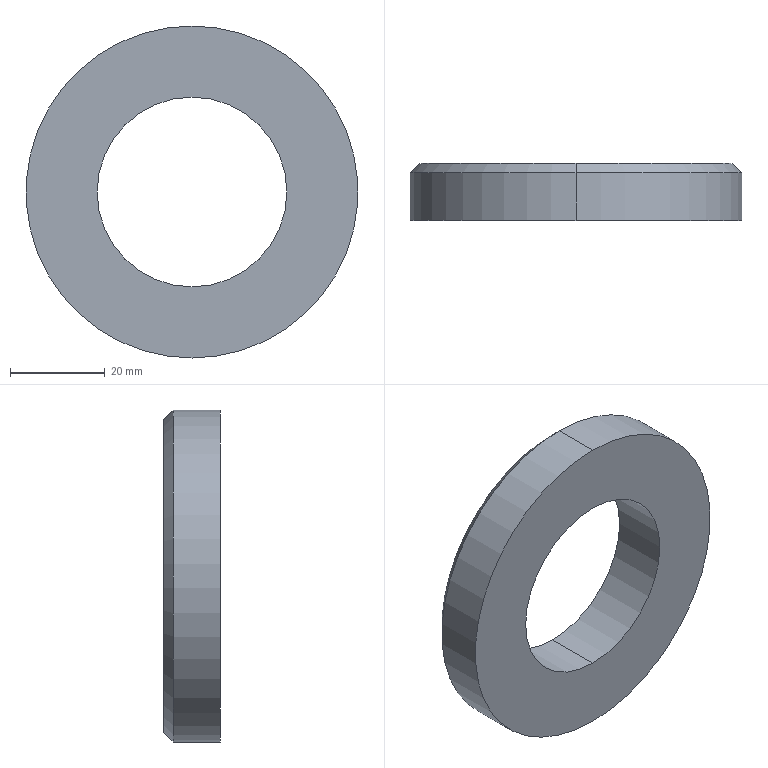Part | SolidWorks | features HoleWzd 1, ICE 1, Revolution 1 | 1 solid | 28 faces | box 70 x 12 x 70 mm | volume 29948 mm3 | cylinder 14 | cone 12 | plane 2 | commonest cylinder face diameters 4.2 x10 40 x2 70 x2
STEP:
#1=CARTESIAN_POINT('',(-27.,2.,-2.1));
#2=VERTEX_POINT('',#1);
#3=CARTESIAN_POINT('',(-27.,2.,2.1));
#4=VERTEX_POINT('',#3);
#5=CARTESIAN_POINT('',(-27.,2.,0.));
#6=DIRECTION('',(0.,1.,0.));
#7=DIRECTION('',(0.,0.,1.));
#8=AXIS2_PLACEMENT_3D('',#5,#6,#7);
#9=CIRCLE('',#8,2.1);
#10=EDGE_CURVE('',#2,#4,#9,.T.);
#11=ORIENTED_EDGE('',*,*,#10,.F.);
#12=CARTESIAN_POINT('',(-27.,12.,-2.1));
#13=VERTEX_POINT('',#12);
#14=CARTESIAN_POINT('',(-27.,12.,-2.1));
#15=DIRECTION('',(0.,1.,0.));
#16=VECTOR('',#15,1000.);
#17=LINE('',#14,#16);
#18=EDGE_CURVE('',#2,#13,#17,.T.);
#19=ORIENTED_EDGE('',*,*,#18,.T.);
#20=CARTESIAN_POINT('',(-27.,12.,2.1));
#21=VERTEX_POINT('',#20);
#22=CARTESIAN_POINT('',(-27.,12.,0.));
#23=DIRECTION('',(0.,1.,0.));
#24=DIRECTION('',(0.,0.,1.));
#25=AXIS2_PLACEMENT_3D('',#22,#23,#24);
#26=CIRCLE('',#25,2.1);
#27=EDGE_CURVE('',#13,#21,#26,.T.);
#28=ORIENTED_EDGE('',*,*,#27,.T.);
#29=CARTESIAN_POINT('',(-27.,12.,2.1));
#30=DIRECTION('',(0.,1.,0.));
#31=VECTOR('',#30,1000.);
#32=LINE('',#29,#31);
#33=EDGE_CURVE('',#4,#21,#32,.T.);
#34=ORIENTED_EDGE('',*,*,#33,.F.);
#35=EDGE_LOOP('',(#11,#19,#28,#34));
#36=FACE_OUTER_BOUND('',#35,.T.);
#37=CARTESIAN_POINT('',(-27.,12.,0.));
#38=DIRECTION('',(0.,1.,0.));
#39=DIRECTION('',(0.,0.,1.));
#40=AXIS2_PLACEMENT_3D('',#37,#38,#39);
#41=CYLINDRICAL_SURFACE('',#40,2.1);
#42=ADVANCED_FACE('',(#36),#41,.F.);
#43=CARTESIAN_POINT('',(-27.,0.7382,0.));
#44=VERTEX_POINT('',#43);
#45=CARTESIAN_POINT('',(-27.,2.,2.1));
#46=DIRECTION('',(0.,0.515,0.8572));
#47=VECTOR('',#46,1000.);
#48=LINE('',#45,#47);
#49=EDGE_CURVE('',#44,#4,#48,.T.);
#50=ORIENTED_EDGE('',*,*,#49,.F.);
#51=CARTESIAN_POINT('',(-27.,2.,-2.1));
#52=DIRECTION('',(0.,0.515,-0.8572));
#53=VECTOR('',#52,1000.);
#54=LINE('',#51,#53);
#55=EDGE_CURVE('',#44,#2,#54,.T.);
#56=ORIENTED_EDGE('',*,*,#55,.T.);
#57=ORIENTED_EDGE('',*,*,#10,.T.);
#58=EDGE_LOOP('',(#50,#56,#57));
#59=FACE_OUTER_BOUND('',#58,.T.);
#60=CARTESIAN_POINT('',(-27.,2.,0.));
#61=DIRECTION('',(0.,1.,0.));
#62=DIRECTION('',(0.,0.,1.));
#63=AXIS2_PLACEMENT_3D('',#60,#61,#62);
#64=CONICAL_SURFACE('',#63,2.1,1.03);
#65=ADVANCED_FACE('',(#59),#64,.F.);
#66=CARTESIAN_POINT('',(-8.343,2.,-27.779));
#67=VERTEX_POINT('',#66);
#68=CARTESIAN_POINT('',(-8.343,2.,-23.579));
#69=VERTEX_POINT('',#68);
#70=CARTESIAN_POINT('',(-8.343,2.,-25.679));
#71=DIRECTION('',(0.,1.,0.));
#72=DIRECTION('',(0.,0.,1.));
#73=AXIS2_PLACEMENT_3D('',#70,#71,#72);
#74=CIRCLE('',#73,2.1);
#75=EDGE_CURVE('',#67,#69,#74,.T.);
#76=ORIENTED_EDGE('',*,*,#75,.F.);
#77=CARTESIAN_POINT('',(-8.343,12.,-27.779));
#78=VERTEX_POINT('',#77);
#79=CARTESIAN_POINT('',(-8.343,12.,-27.779));
#80=DIRECTION('',(0.,1.,0.));
#81=VECTOR('',#80,1000.);
#82=LINE('',#79,#81);
#83=EDGE_CURVE('',#67,#78,#82,.T.);
#84=ORIENTED_EDGE('',*,*,#83,.T.);
#85=CARTESIAN_POINT('',(-8.343,12.,-23.579));
#86=VERTEX_POINT('',#85);
#87=CARTESIAN_POINT('',(-8.343,12.,-25.679));
#88=DIRECTION('',(0.,1.,0.));
#89=DIRECTION('',(0.,0.,1.));
#90=AXIS2_PLACEMENT_3D('',#87,#88,#89);
#91=CIRCLE('',#90,2.1);
#92=EDGE_CURVE('',#78,#86,#91,.T.);
#93=ORIENTED_EDGE('',*,*,#92,.T.);
#94=CARTESIAN_POINT('',(-8.343,12.,-23.579));
#95=DIRECTION('',(0.,1.,0.));
#96=VECTOR('',#95,1000.);
#97=LINE('',#94,#96);
#98=EDGE_CURVE('',#69,#86,#97,.T.);
#99=ORIENTED_EDGE('',*,*,#98,.F.);
#100=EDGE_LOOP('',(#76,#84,#93,#99));
#101=FACE_OUTER_BOUND('',#100,.T.);
#102=CARTESIAN_POINT('',(-8.343,12.,-25.679));
#103=DIRECTION('',(0.,1.,0.));
#104=DIRECTION('',(0.,0.,1.));
#105=AXIS2_PLACEMENT_3D('',#102,#103,#104);
#106=CYLINDRICAL_SURFACE('',#105,2.1);
#107=ADVANCED_FACE('',(#101),#106,.F.);
#108=CARTESIAN_POINT('',(-8.343,0.7382,-25.679));
#109=VERTEX_POINT('',#108);
#110=CARTESIAN_POINT('',(-8.343,2.,-23.579));
#111=DIRECTION('',(0.,0.515,0.8572));
#112=VECTOR('',#111,1000.);
#113=LINE('',#110,#112);
#114=EDGE_CURVE('',#109,#69,#113,.T.);
#115=ORIENTED_EDGE('',*,*,#114,.F.);
#116=CARTESIAN_POINT('',(-8.343,2.,-27.779));
#117=DIRECTION('',(0.,0.515,-0.8572));
#118=VECTOR('',#117,1000.);
#119=LINE('',#116,#118);
#120=EDGE_CURVE('',#109,#67,#119,.T.);
#121=ORIENTED_EDGE('',*,*,#120,.T.);
#122=ORIENTED_EDGE('',*,*,#75,.T.);
#123=EDGE_LOOP('',(#115,#121,#122));
#124=FACE_OUTER_BOUND('',#123,.T.);
#125=CARTESIAN_POINT('',(-8.343,2.,-25.679));
#126=DIRECTION('',(0.,1.,0.));
#127=DIRECTION('',(0.,0.,1.));
#128=AXIS2_PLACEMENT_3D('',#125,#126,#127);
#129=CONICAL_SURFACE('',#128,2.1,1.03);
#130=ADVANCED_FACE('',(#124),#129,.F.);
#131=CARTESIAN_POINT('',(20.683,2.,-19.455));
#132=VERTEX_POINT('',#131);
#133=CARTESIAN_POINT('',(20.683,2.,-15.255));
#134=VERTEX_POINT('',#133);
#135=CARTESIAN_POINT('',(20.683,2.,-17.355));
#136=DIRECTION('',(0.,1.,0.));
#137=DIRECTION('',(0.,0.,1.));
#138=AXIS2_PLACEMENT_3D('',#135,#136,#137);
#139=CIRCLE('',#138,2.1);
#140=EDGE_CURVE('',#132,#134,#139,.T.);
#141=ORIENTED_EDGE('',*,*,#140,.F.);
#142=CARTESIAN_POINT('',(20.683,12.,-19.455));
#143=VERTEX_POINT('',#142);
#144=CARTESIAN_POINT('',(20.683,12.,-19.455));
#145=DIRECTION('',(0.,1.,0.));
#146=VECTOR('',#145,1000.);
#147=LINE('',#144,#146);
#148=EDGE_CURVE('',#132,#143,#147,.T.);
#149=ORIENTED_EDGE('',*,*,#148,.T.);
#150=CARTESIAN_POINT('',(20.683,12.,-15.255));
#151=VERTEX_POINT('',#150);
#152=CARTESIAN_POINT('',(20.683,12.,-17.355));
#153=DIRECTION('',(0.,1.,0.));
#154=DIRECTION('',(0.,0.,1.));
#155=AXIS2_PLACEMENT_3D('',#152,#153,#154);
#156=CIRCLE('',#155,2.1);
#157=EDGE_CURVE('',#143,#151,#156,.T.);
#158=ORIENTED_EDGE('',*,*,#157,.T.);
#159=CARTESIAN_POINT('',(20.683,12.,-15.255));
#160=DIRECTION('',(0.,1.,0.));
#161=VECTOR('',#160,1000.);
#162=LINE('',#159,#161);
#163=EDGE_CURVE('',#134,#151,#162,.T.);
#164=ORIENTED_EDGE('',*,*,#163,.F.);
#165=EDGE_LOOP('',(#141,#149,#158,#164));
#166=FACE_OUTER_BOUND('',#165,.T.);
#167=CARTESIAN_POINT('',(20.683,12.,-17.355));
#168=DIRECTION('',(0.,1.,0.));
#169=DIRECTION('',(0.,0.,1.));
#170=AXIS2_PLACEMENT_3D('',#167,#168,#169);
#171=CYLINDRICAL_SURFACE('',#170,2.1);
#172=ADVANCED_FACE('',(#166),#171,.F.);
#173=CARTESIAN_POINT('',(20.683,0.7382,-17.355));
#174=VERTEX_POINT('',#173);
#175=CARTESIAN_POINT('',(20.683,2.,-15.255));
#176=DIRECTION('',(0.,0.515,0.8572));
#177=VECTOR('',#176,1000.);
#178=LINE('',#175,#177);
#179=EDGE_CURVE('',#174,#134,#178,.T.);
#180=ORIENTED_EDGE('',*,*,#179,.F.);
#181=CARTESIAN_POINT('',(20.683,2.,-19.455));
#182=DIRECTION('',(0.,0.515,-0.8572));
#183=VECTOR('',#182,1000.);
#184=LINE('',#181,#183);
#185=EDGE_CURVE('',#174,#132,#184,.T.);
#186=ORIENTED_EDGE('',*,*,#185,.T.);
#187=ORIENTED_EDGE('',*,*,#140,.T.);
#188=EDGE_LOOP('',(#180,#186,#187));
#189=FACE_OUTER_BOUND('',#188,.T.);
#190=CARTESIAN_POINT('',(20.683,2.,-17.355));
#191=DIRECTION('',(0.,1.,0.));
#192=DIRECTION('',(0.,0.,1.));
#193=AXIS2_PLACEMENT_3D('',#190,#191,#192);
#194=CONICAL_SURFACE('',#193,2.1,1.03);
#195=ADVANCED_FACE('',(#189),#194,.F.);
#196=CARTESIAN_POINT('',(20.683,2.,15.255));
#197=VERTEX_POINT('',#196);
#198=CARTESIAN_POINT('',(20.683,2.,19.455));
#199=VERTEX_POINT('',#198);
#200=CARTESIAN_POINT('',(20.683,2.,17.355));
#201=DIRECTION('',(0.,1.,0.));
#202=DIRECTION('',(0.,0.,1.));
#203=AXIS2_PLACEMENT_3D('',#200,#201,#202);
#204=CIRCLE('',#203,2.1);
#205=EDGE_CURVE('',#197,#199,#204,.T.);
#206=ORIENTED_EDGE('',*,*,#205,.F.);
#207=CARTESIAN_POINT('',(20.683,12.,15.255));
#208=VERTEX_POINT('',#207);
#209=CARTESIAN_POINT('',(20.683,12.,15.255));
#210=DIRECTION('',(0.,1.,0.));
#211=VECTOR('',#210,1000.);
#212=LINE('',#209,#211);
#213=EDGE_CURVE('',#197,#208,#212,.T.);
#214=ORIENTED_EDGE('',*,*,#213,.T.);
#215=CARTESIAN_POINT('',(20.683,12.,19.455));
#216=VERTEX_POINT('',#215);
#217=CARTESIAN_POINT('',(20.683,12.,17.355));
#218=DIRECTION('',(0.,1.,0.));
#219=DIRECTION('',(0.,0.,1.));
#220=AXIS2_PLACEMENT_3D('',#217,#218,#219);
#221=CIRCLE('',#220,2.1);
#222=EDGE_CURVE('',#208,#216,#221,.T.);
#223=ORIENTED_EDGE('',*,*,#222,.T.);
#224=CARTESIAN_POINT('',(20.683,12.,19.455));
#225=DIRECTION('',(0.,1.,0.));
#226=VECTOR('',#225,1000.);
#227=LINE('',#224,#226);
#228=EDGE_CURVE('',#199,#216,#227,.T.);
#229=ORIENTED_EDGE('',*,*,#228,.F.);
#230=EDGE_LOOP('',(#206,#214,#223,#229));
#231=FACE_OUTER_BOUND('',#230,.T.);
#232=CARTESIAN_POINT('',(20.683,12.,17.355));
#233=DIRECTION('',(0.,1.,0.));
#234=DIRECTION('',(0.,0.,1.));
#235=AXIS2_PLACEMENT_3D('',#232,#233,#234);
#236=CYLINDRICAL_SURFACE('',#235,2.1);
#237=ADVANCED_FACE('',(#231),#236,.F.);
#238=CARTESIAN_POINT('',(20.683,0.7382,17.355));
#239=VERTEX_POINT('',#238);
#240=CARTESIAN_POINT('',(20.683,2.,19.455));
#241=DIRECTION('',(0.,0.515,0.8572));
#242=VECTOR('',#241,1000.);
#243=LINE('',#240,#242);
#244=EDGE_CURVE('',#239,#199,#243,.T.);
#245=ORIENTED_EDGE('',*,*,#244,.F.);
#246=CARTESIAN_POINT('',(20.683,2.,15.255));
#247=DIRECTION('',(0.,0.515,-0.8572));
#248=VECTOR('',#247,1000.);
#249=LINE('',#246,#248);
#250=EDGE_CURVE('',#239,#197,#249,.T.);
#251=ORIENTED_EDGE('',*,*,#250,.T.);
#252=ORIENTED_EDGE('',*,*,#205,.T.);
#253=EDGE_LOOP('',(#245,#251,#252));
#254=FACE_OUTER_BOUND('',#253,.T.);
#255=CARTESIAN_POINT('',(20.683,2.,17.355));
#256=DIRECTION('',(0.,1.,0.));
#257=DIRECTION('',(0.,0.,1.));
#258=AXIS2_PLACEMENT_3D('',#255,#256,#257);
#259=CONICAL_SURFACE('',#258,2.1,1.03);
#260=ADVANCED_FACE('',(#254),#259,.F.);
#261=CARTESIAN_POINT('',(-8.343,2.,23.579));
#262=VERTEX_POINT('',#261);
#263=CARTESIAN_POINT('',(-8.343,2.,27.779));
#264=VERTEX_POINT('',#263);
#265=CARTESIAN_POINT('',(-8.343,2.,25.679));
#266=DIRECTION('',(0.,1.,0.));
#267=DIRECTION('',(0.,0.,1.));
#268=AXIS2_PLACEMENT_3D('',#265,#266,#267);
#269=CIRCLE('',#268,2.1);
#270=EDGE_CURVE('',#262,#264,#269,.T.);
#271=ORIENTED_EDGE('',*,*,#270,.F.);
#272=CARTESIAN_POINT('',(-8.343,12.,23.579));
#273=VERTEX_POINT('',#272);
#274=CARTESIAN_POINT('',(-8.343,12.,23.579));
#275=DIRECTION('',(0.,1.,0.));
#276=VECTOR('',#275,1000.);
#277=LINE('',#274,#276);
#278=EDGE_CURVE('',#262,#273,#277,.T.);
#279=ORIENTED_EDGE('',*,*,#278,.T.);
#280=CARTESIAN_POINT('',(-8.343,12.,27.779));
#281=VERTEX_POINT('',#280);
#282=CARTESIAN_POINT('',(-8.343,12.,25.679));
#283=DIRECTION('',(0.,1.,0.));
#284=DIRECTION('',(0.,0.,1.));
#285=AXIS2_PLACEMENT_3D('',#282,#283,#284);
#286=CIRCLE('',#285,2.1);
#287=EDGE_CURVE('',#273,#281,#286,.T.);
#288=ORIENTED_EDGE('',*,*,#287,.T.);
#289=CARTESIAN_POINT('',(-8.343,12.,27.779));
#290=DIRECTION('',(0.,1.,0.));
#291=VECTOR('',#290,1000.);
#292=LINE('',#289,#291);
#293=EDGE_CURVE('',#264,#281,#292,.T.);
#294=ORIENTED_EDGE('',*,*,#293,.F.);
#295=EDGE_LOOP('',(#271,#279,#288,#294));
#296=FACE_OUTER_BOUND('',#295,.T.);
#297=CARTESIAN_POINT('',(-8.343,12.,25.679));
#298=DIRECTION('',(0.,1.,0.));
#299=DIRECTION('',(0.,0.,1.));
#300=AXIS2_PLACEMENT_3D('',#297,#298,#299);
#301=CYLINDRICAL_SURFACE('',#300,2.1);
#302=ADVANCED_FACE('',(#296),#301,.F.);
#303=CARTESIAN_POINT('',(-8.343,0.7382,25.679));
#304=VERTEX_POINT('',#303);
#305=CARTESIAN_POINT('',(-8.343,2.,27.779));
#306=DIRECTION('',(0.,0.515,0.8572));
#307=VECTOR('',#306,1000.);
#308=LINE('',#305,#307);
#309=EDGE_CURVE('',#304,#264,#308,.T.);
#310=ORIENTED_EDGE('',*,*,#309,.F.);
#311=CARTESIAN_POINT('',(-8.343,2.,23.579));
#312=DIRECTION('',(0.,0.515,-0.8572));
#313=VECTOR('',#312,1000.);
#314=LINE('',#311,#313);
#315=EDGE_CURVE('',#304,#262,#314,.T.);
#316=ORIENTED_EDGE('',*,*,#315,.T.);
#317=ORIENTED_EDGE('',*,*,#270,.T.);
#318=EDGE_LOOP('',(#310,#316,#317));
#319=FACE_OUTER_BOUND('',#318,.T.);
#320=CARTESIAN_POINT('',(-8.343,2.,25.679));
#321=DIRECTION('',(0.,1.,0.));
#322=DIRECTION('',(0.,0.,1.));
#323=AXIS2_PLACEMENT_3D('',#320,#321,#322);
#324=CONICAL_SURFACE('',#323,2.1,1.03);
#325=ADVANCED_FACE('',(#319),#324,.F.);
#326=CARTESIAN_POINT('',(0.,12.,-33.));
#327=VERTEX_POINT('',#326);
#328=CARTESIAN_POINT('',(0.,12.,33.));
#329=VERTEX_POINT('',#328);
#330=CARTESIAN_POINT('',(0.,12.,0.));
#331=DIRECTION('',(0.,-1.,0.));
#332=DIRECTION('',(0.,0.,-1.));
#333=AXIS2_PLACEMENT_3D('',#330,#331,#332);
#334=CIRCLE('',#333,33.);
#335=EDGE_CURVE('',#327,#329,#334,.T.);
#336=ORIENTED_EDGE('',*,*,#335,.T.);
#337=CARTESIAN_POINT('',(0.,10.,35.));
#338=VERTEX_POINT('',#337);
#339=CARTESIAN_POINT('',(0.,10.,35.));
#340=DIRECTION('',(0.,-0.7071,0.7071));
#341=VECTOR('',#340,1000.);
#342=LINE('',#339,#341);
#343=EDGE_CURVE('',#329,#338,#342,.T.);
#344=ORIENTED_EDGE('',*,*,#343,.T.);
#345=CARTESIAN_POINT('',(0.,10.,-35.));
#346=VERTEX_POINT('',#345);
#347=CARTESIAN_POINT('',(0.,10.,0.));
#348=DIRECTION('',(0.,-1.,0.));
#349=DIRECTION('',(0.,0.,-1.));
#350=AXIS2_PLACEMENT_3D('',#347,#348,#349);
#351=CIRCLE('',#350,35.);
#352=EDGE_CURVE('',#346,#338,#351,.T.);
#353=ORIENTED_EDGE('',*,*,#352,.F.);
#354=CARTESIAN_POINT('',(0.,10.,-35.));
#355=DIRECTION('',(0.,-0.7071,-0.7071));
#356=VECTOR('',#355,1000.);
#357=LINE('',#354,#356);
#358=EDGE_CURVE('',#327,#346,#357,.T.);
#359=ORIENTED_EDGE('',*,*,#358,.F.);
#360=EDGE_LOOP('',(#336,#344,#353,#359));
#361=FACE_OUTER_BOUND('',#360,.T.);
#362=CARTESIAN_POINT('',(0.,10.,0.));
#363=DIRECTION('',(0.,-1.,0.));
#364=DIRECTION('',(0.,0.,-1.));
#365=AXIS2_PLACEMENT_3D('',#362,#363,#364);
#366=CONICAL_SURFACE('',#365,35.,0.7854);
#367=ADVANCED_FACE('',(#361),#366,.T.);
#368=ORIENTED_EDGE('',*,*,#352,.T.);
#369=CARTESIAN_POINT('',(0.,0.,35.));
#370=VERTEX_POINT('',#369);
#371=CARTESIAN_POINT('',(0.,0.,35.));
#372=DIRECTION('',(0.,-1.,0.));
#373=VECTOR('',#372,1000.);
#374=LINE('',#371,#373);
#375=EDGE_CURVE('',#338,#370,#374,.T.);
#376=ORIENTED_EDGE('',*,*,#375,.T.);
#377=CARTESIAN_POINT('',(0.,0.,-35.));
#378=VERTEX_POINT('',#377);
#379=CARTESIAN_POINT('',(0.,0.,0.));
#380=DIRECTION('',(0.,-1.,0.));
#381=DIRECTION('',(0.,0.,-1.));
#382=AXIS2_PLACEMENT_3D('',#379,#380,#381);
#383=CIRCLE('',#382,35.);
#384=EDGE_CURVE('',#378,#370,#383,.T.);
#385=ORIENTED_EDGE('',*,*,#384,.F.);
#386=CARTESIAN_POINT('',(0.,0.,-35.));
#387=DIRECTION('',(0.,-1.,0.));
#388=VECTOR('',#387,1000.);
#389=LINE('',#386,#388);
#390=EDGE_CURVE('',#346,#378,#389,.T.);
#391=ORIENTED_EDGE('',*,*,#390,.F.);
#392=EDGE_LOOP('',(#368,#376,#385,#391));
#393=FACE_OUTER_BOUND('',#392,.T.);
#394=CARTESIAN_POINT('',(0.,0.,0.));
#395=DIRECTION('',(0.,-1.,0.));
#396=DIRECTION('',(0.,0.,-1.));
#397=AXIS2_PLACEMENT_3D('',#394,#395,#396);
#398=CYLINDRICAL_SURFACE('',#397,35.);
#399=ADVANCED_FACE('',(#393),#398,.T.);
#400=CARTESIAN_POINT('',(0.,12.,20.));
#401=VERTEX_POINT('',#400);
#402=CARTESIAN_POINT('',(0.,12.,-20.));
#403=VERTEX_POINT('',#402);
#404=CARTESIAN_POINT('',(0.,12.,0.));
#405=DIRECTION('',(0.,-1.,0.));
#406=DIRECTION('',(0.,0.,-1.));
#407=AXIS2_PLACEMENT_3D('',#404,#405,#406);
#408=CIRCLE('',#407,20.);
#409=EDGE_CURVE('',#401,#403,#408,.T.);
#410=ORIENTED_EDGE('',*,*,#409,.F.);
#411=CARTESIAN_POINT('',(0.,0.,20.));
#412=VERTEX_POINT('',#411);
#413=CARTESIAN_POINT('',(0.,0.,20.));
#414=DIRECTION('',(0.,-1.,0.));
#415=VECTOR('',#414,1000.);
#416=LINE('',#413,#415);
#417=EDGE_CURVE('',#401,#412,#416,.T.);
#418=ORIENTED_EDGE('',*,*,#417,.T.);
#419=CARTESIAN_POINT('',(0.,0.,-20.));
#420=VERTEX_POINT('',#419);
#421=CARTESIAN_POINT('',(0.,0.,0.));
#422=DIRECTION('',(0.,-1.,0.));
#423=DIRECTION('',(0.,0.,-1.));
#424=AXIS2_PLACEMENT_3D('',#421,#422,#423);
#425=CIRCLE('',#424,20.);
#426=EDGE_CURVE('',#412,#420,#425,.T.);
#427=ORIENTED_EDGE('',*,*,#426,.T.);
#428=CARTESIAN_POINT('',(0.,0.,-20.));
#429=DIRECTION('',(0.,-1.,0.));
#430=VECTOR('',#429,1000.);
#431=LINE('',#428,#430);
#432=EDGE_CURVE('',#403,#420,#431,.T.);
#433=ORIENTED_EDGE('',*,*,#432,.F.);
#434=EDGE_LOOP('',(#410,#418,#427,#433));
#435=FACE_OUTER_BOUND('',#434,.T.);
#436=CARTESIAN_POINT('',(0.,0.,0.));
#437=DIRECTION('',(0.,-1.,0.));
#438=DIRECTION('',(0.,0.,-1.));
#439=AXIS2_PLACEMENT_3D('',#436,#437,#438);
#440=CYLINDRICAL_SURFACE('',#439,20.);
#441=ADVANCED_FACE('',(#435),#440,.F.);
#442=ORIENTED_EDGE('',*,*,#417,.F.);
#443=CARTESIAN_POINT('',(0.,12.,0.));
#444=DIRECTION('',(0.,-1.,0.));
#445=DIRECTION('',(0.,0.,-1.));
#446=AXIS2_PLACEMENT_3D('',#443,#444,#445);
#447=CIRCLE('',#446,20.);
#448=EDGE_CURVE('',#403,#401,#447,.T.);
#449=ORIENTED_EDGE('',*,*,#448,.F.);
#450=ORIENTED_EDGE('',*,*,#432,.T.);
#451=CARTESIAN_POINT('',(0.,0.,0.));
#452=DIRECTION('',(0.,-1.,0.));
#453=DIRECTION('',(0.,0.,-1.));
#454=AXIS2_PLACEMENT_3D('',#451,#452,#453);
#455=CIRCLE('',#454,20.);
#456=EDGE_CURVE('',#420,#412,#455,.T.);
#457=ORIENTED_EDGE('',*,*,#456,.T.);
#458=EDGE_LOOP('',(#442,#449,#450,#457));
#459=FACE_OUTER_BOUND('',#458,.T.);
#460=CARTESIAN_POINT('',(0.,0.,0.));
#461=DIRECTION('',(0.,-1.,0.));
#462=DIRECTION('',(0.,0.,-1.));
#463=AXIS2_PLACEMENT_3D('',#460,#461,#462);
#464=CYLINDRICAL_SURFACE('',#463,20.);
#465=ADVANCED_FACE('',(#459),#464,.F.);
#466=ORIENTED_EDGE('',*,*,#384,.T.);
#467=CARTESIAN_POINT('',(0.,0.,0.));
#468=DIRECTION('',(0.,-1.,0.));
#469=DIRECTION('',(0.,0.,-1.));
#470=AXIS2_PLACEMENT_3D('',#467,#468,#469);
#471=CIRCLE('',#470,35.);
#472=EDGE_CURVE('',#370,#378,#471,.T.);
#473=ORIENTED_EDGE('',*,*,#472,.T.);
#474=EDGE_LOOP('',(#466,#473));
#475=FACE_OUTER_BOUND('',#474,.T.);
#476=ORIENTED_EDGE('',*,*,#456,.F.);
#477=ORIENTED_EDGE('',*,*,#426,.F.);
#478=EDGE_LOOP('',(#476,#477));
#479=FACE_BOUND('',#478,.T.);
#480=CARTESIAN_POINT('',(0.,0.,-20.));
#481=DIRECTION('',(0.,-1.,0.));
#482=DIRECTION('',(0.,0.,-1.));
#483=AXIS2_PLACEMENT_3D('',#480,#481,#482);
#484=PLANE('',#483);
#485=ADVANCED_FACE('',(#475,#479),#484,.T.);
#486=ORIENTED_EDGE('',*,*,#375,.F.);
#487=CARTESIAN_POINT('',(0.,10.,0.));
#488=DIRECTION('',(0.,-1.,0.));
#489=DIRECTION('',(0.,0.,-1.));
#490=AXIS2_PLACEMENT_3D('',#487,#488,#489);
#491=CIRCLE('',#490,35.);
#492=EDGE_CURVE('',#338,#346,#491,.T.);
#493=ORIENTED_EDGE('',*,*,#492,.T.);
#494=ORIENTED_EDGE('',*,*,#390,.T.);
#495=ORIENTED_EDGE('',*,*,#472,.F.);
#496=EDGE_LOOP('',(#486,#493,#494,#495));
#497=FACE_OUTER_BOUND('',#496,.T.);
#498=CARTESIAN_POINT('',(0.,0.,0.));
#499=DIRECTION('',(0.,-1.,0.));
#500=DIRECTION('',(0.,0.,-1.));
#501=AXIS2_PLACEMENT_3D('',#498,#499,#500);
#502=CYLINDRICAL_SURFACE('',#501,35.);
#503=ADVANCED_FACE('',(#497),#502,.T.);
#504=ORIENTED_EDGE('',*,*,#343,.F.);
#505=CARTESIAN_POINT('',(0.,12.,0.));
#506=DIRECTION('',(0.,-1.,0.));
#507=DIRECTION('',(0.,0.,-1.));
#508=AXIS2_PLACEMENT_3D('',#505,#506,#507);
#509=CIRCLE('',#508,33.);
#510=EDGE_CURVE('',#329,#327,#509,.T.);
#511=ORIENTED_EDGE('',*,*,#510,.T.);
#512=ORIENTED_EDGE('',*,*,#358,.T.);
#513=ORIENTED_EDGE('',*,*,#492,.F.);
#514=EDGE_LOOP('',(#504,#511,#512,#513));
#515=FACE_OUTER_BOUND('',#514,.T.);
#516=CARTESIAN_POINT('',(0.,10.,0.));
#517=DIRECTION('',(0.,-1.,0.));
#518=DIRECTION('',(0.,0.,-1.));
#519=AXIS2_PLACEMENT_3D('',#516,#517,#518);
#520=CONICAL_SURFACE('',#519,35.,0.7854);
#521=ADVANCED_FACE('',(#515),#520,.T.);
#522=CARTESIAN_POINT('',(-27.,12.,0.));
#523=DIRECTION('',(0.,1.,0.));
#524=DIRECTION('',(0.,0.,1.));
#525=AXIS2_PLACEMENT_3D('',#522,#523,#524);
#526=CIRCLE('',#525,2.1);
#527=EDGE_CURVE('',#21,#13,#526,.T.);
#528=ORIENTED_EDGE('',*,*,#527,.F.);
#529=ORIENTED_EDGE('',*,*,#27,.F.);
#530=EDGE_LOOP('',(#528,#529));
#531=FACE_BOUND('',#530,.T.);
#532=CARTESIAN_POINT('',(-8.343,12.,-25.679));
#533=DIRECTION('',(0.,1.,0.));
#534=DIRECTION('',(0.,0.,1.));
#535=AXIS2_PLACEMENT_3D('',#532,#533,#534);
#536=CIRCLE('',#535,2.1);
#537=EDGE_CURVE('',#86,#78,#536,.T.);
#538=ORIENTED_EDGE('',*,*,#537,.F.);
#539=ORIENTED_EDGE('',*,*,#92,.F.);
#540=EDGE_LOOP('',(#538,#539));
#541=FACE_BOUND('',#540,.T.);
#542=CARTESIAN_POINT('',(20.683,12.,-17.355));
#543=DIRECTION('',(0.,1.,0.));
#544=DIRECTION('',(0.,0.,1.));
#545=AXIS2_PLACEMENT_3D('',#542,#543,#544);
#546=CIRCLE('',#545,2.1);
#547=EDGE_CURVE('',#151,#143,#546,.T.);
#548=ORIENTED_EDGE('',*,*,#547,.F.);
#549=ORIENTED_EDGE('',*,*,#157,.F.);
#550=EDGE_LOOP('',(#548,#549));
#551=FACE_BOUND('',#550,.T.);
#552=CARTESIAN_POINT('',(20.683,12.,17.355));
#553=DIRECTION('',(0.,1.,0.));
#554=DIRECTION('',(0.,0.,1.));
#555=AXIS2_PLACEMENT_3D('',#552,#553,#554);
#556=CIRCLE('',#555,2.1);
#557=EDGE_CURVE('',#216,#208,#556,.T.);
#558=ORIENTED_EDGE('',*,*,#557,.F.);
#559=ORIENTED_EDGE('',*,*,#222,.F.);
#560=EDGE_LOOP('',(#558,#559));
#561=FACE_BOUND('',#560,.T.);
#562=CARTESIAN_POINT('',(-8.343,12.,25.679));
#563=DIRECTION('',(0.,1.,0.));
#564=DIRECTION('',(0.,0.,1.));
#565=AXIS2_PLACEMENT_3D('',#562,#563,#564);
#566=CIRCLE('',#565,2.1);
#567=EDGE_CURVE('',#281,#273,#566,.T.);
#568=ORIENTED_EDGE('',*,*,#567,.F.);
#569=ORIENTED_EDGE('',*,*,#287,.F.);
#570=EDGE_LOOP('',(#568,#569));
#571=FACE_BOUND('',#570,.T.);
#572=ORIENTED_EDGE('',*,*,#448,.T.);
#573=ORIENTED_EDGE('',*,*,#409,.T.);
#574=EDGE_LOOP('',(#572,#573));
#575=FACE_BOUND('',#574,.T.);
#576=ORIENTED_EDGE('',*,*,#335,.F.);
#577=ORIENTED_EDGE('',*,*,#510,.F.);
#578=EDGE_LOOP('',(#576,#577));
#579=FACE_OUTER_BOUND('',#578,.T.);
#580=CARTESIAN_POINT('',(0.,12.,-33.));
#581=DIRECTION('',(0.,1.,0.));
#582=DIRECTION('',(0.,0.,1.));
#583=AXIS2_PLACEMENT_3D('',#580,#581,#582);
#584=PLANE('',#583);
#585=ADVANCED_FACE('',(#531,#541,#551,#561,#571,#575,#579),#584,.T.);
#586=ORIENTED_EDGE('',*,*,#315,.F.);
#587=ORIENTED_EDGE('',*,*,#309,.T.);
#588=CARTESIAN_POINT('',(-8.343,2.,25.679));
#589=DIRECTION('',(0.,1.,0.));
#590=DIRECTION('',(0.,0.,1.));
#591=AXIS2_PLACEMENT_3D('',#588,#589,#590);
#592=CIRCLE('',#591,2.1);
#593=EDGE_CURVE('',#264,#262,#592,.T.);
#594=ORIENTED_EDGE('',*,*,#593,.T.);
#595=EDGE_LOOP('',(#586,#587,#594));
#596=FACE_OUTER_BOUND('',#595,.T.);
#597=CARTESIAN_POINT('',(-8.343,2.,25.679));
#598=DIRECTION('',(0.,1.,0.));
#599=DIRECTION('',(0.,0.,1.));
#600=AXIS2_PLACEMENT_3D('',#597,#598,#599);
#601=CONICAL_SURFACE('',#600,2.1,1.03);
#602=ADVANCED_FACE('',(#596),#601,.F.);
#603=ORIENTED_EDGE('',*,*,#278,.F.);
#604=ORIENTED_EDGE('',*,*,#593,.F.);
#605=ORIENTED_EDGE('',*,*,#293,.T.);
#606=ORIENTED_EDGE('',*,*,#567,.T.);
#607=EDGE_LOOP('',(#603,#604,#605,#606));
#608=FACE_OUTER_BOUND('',#607,.T.);
#609=CARTESIAN_POINT('',(-8.343,12.,25.679));
#610=DIRECTION('',(0.,1.,0.));
#611=DIRECTION('',(0.,0.,1.));
#612=AXIS2_PLACEMENT_3D('',#609,#610,#611);
#613=CYLINDRICAL_SURFACE('',#612,2.1);
#614=ADVANCED_FACE('',(#608),#613,.F.);
#615=ORIENTED_EDGE('',*,*,#250,.F.);
#616=ORIENTED_EDGE('',*,*,#244,.T.);
#617=CARTESIAN_POINT('',(20.683,2.,17.355));
#618=DIRECTION('',(0.,1.,0.));
#619=DIRECTION('',(0.,0.,1.));
#620=AXIS2_PLACEMENT_3D('',#617,#618,#619);
#621=CIRCLE('',#620,2.1);
#622=EDGE_CURVE('',#199,#197,#621,.T.);
#623=ORIENTED_EDGE('',*,*,#622,.T.);
#624=EDGE_LOOP('',(#615,#616,#623));
#625=FACE_OUTER_BOUND('',#624,.T.);
#626=CARTESIAN_POINT('',(20.683,2.,17.355));
#627=DIRECTION('',(0.,1.,0.));
#628=DIRECTION('',(0.,0.,1.));
#629=AXIS2_PLACEMENT_3D('',#626,#627,#628);
#630=CONICAL_SURFACE('',#629,2.1,1.03);
#631=ADVANCED_FACE('',(#625),#630,.F.);
#632=ORIENTED_EDGE('',*,*,#213,.F.);
#633=ORIENTED_EDGE('',*,*,#622,.F.);
#634=ORIENTED_EDGE('',*,*,#228,.T.);
#635=ORIENTED_EDGE('',*,*,#557,.T.);
#636=EDGE_LOOP('',(#632,#633,#634,#635));
#637=FACE_OUTER_BOUND('',#636,.T.);
#638=CARTESIAN_POINT('',(20.683,12.,17.355));
#639=DIRECTION('',(0.,1.,0.));
#640=DIRECTION('',(0.,0.,1.));
#641=AXIS2_PLACEMENT_3D('',#638,#639,#640);
#642=CYLINDRICAL_SURFACE('',#641,2.1);
#643=ADVANCED_FACE('',(#637),#642,.F.);
#644=ORIENTED_EDGE('',*,*,#185,.F.);
#645=ORIENTED_EDGE('',*,*,#179,.T.);
#646=CARTESIAN_POINT('',(20.683,2.,-17.355));
#647=DIRECTION('',(0.,1.,0.));
#648=DIRECTION('',(0.,0.,1.));
#649=AXIS2_PLACEMENT_3D('',#646,#647,#648);
#650=CIRCLE('',#649,2.1);
#651=EDGE_CURVE('',#134,#132,#650,.T.);
#652=ORIENTED_EDGE('',*,*,#651,.T.);
#653=EDGE_LOOP('',(#644,#645,#652));
#654=FACE_OUTER_BOUND('',#653,.T.);
#655=CARTESIAN_POINT('',(20.683,2.,-17.355));
#656=DIRECTION('',(0.,1.,0.));
#657=DIRECTION('',(0.,0.,1.));
#658=AXIS2_PLACEMENT_3D('',#655,#656,#657);
#659=CONICAL_SURFACE('',#658,2.1,1.03);
#660=ADVANCED_FACE('',(#654),#659,.F.);
#661=ORIENTED_EDGE('',*,*,#148,.F.);
#662=ORIENTED_EDGE('',*,*,#651,.F.);
#663=ORIENTED_EDGE('',*,*,#163,.T.);
#664=ORIENTED_EDGE('',*,*,#547,.T.);
#665=EDGE_LOOP('',(#661,#662,#663,#664));
#666=FACE_OUTER_BOUND('',#665,.T.);
#667=CARTESIAN_POINT('',(20.683,12.,-17.355));
#668=DIRECTION('',(0.,1.,0.));
#669=DIRECTION('',(0.,0.,1.));
#670=AXIS2_PLACEMENT_3D('',#667,#668,#669);
#671=CYLINDRICAL_SURFACE('',#670,2.1);
#672=ADVANCED_FACE('',(#666),#671,.F.);
#673=ORIENTED_EDGE('',*,*,#120,.F.);
#674=ORIENTED_EDGE('',*,*,#114,.T.);
#675=CARTESIAN_POINT('',(-8.343,2.,-25.679));
#676=DIRECTION('',(0.,1.,0.));
#677=DIRECTION('',(0.,0.,1.));
#678=AXIS2_PLACEMENT_3D('',#675,#676,#677);
#679=CIRCLE('',#678,2.1);
#680=EDGE_CURVE('',#69,#67,#679,.T.);
#681=ORIENTED_EDGE('',*,*,#680,.T.);
#682=EDGE_LOOP('',(#673,#674,#681));
#683=FACE_OUTER_BOUND('',#682,.T.);
#684=CARTESIAN_POINT('',(-8.343,2.,-25.679));
#685=DIRECTION('',(0.,1.,0.));
#686=DIRECTION('',(0.,0.,1.));
#687=AXIS2_PLACEMENT_3D('',#684,#685,#686);
#688=CONICAL_SURFACE('',#687,2.1,1.03);
#689=ADVANCED_FACE('',(#683),#688,.F.);
#690=ORIENTED_EDGE('',*,*,#83,.F.);
#691=ORIENTED_EDGE('',*,*,#680,.F.);
#692=ORIENTED_EDGE('',*,*,#98,.T.);
#693=ORIENTED_EDGE('',*,*,#537,.T.);
#694=EDGE_LOOP('',(#690,#691,#692,#693));
#695=FACE_OUTER_BOUND('',#694,.T.);
#696=CARTESIAN_POINT('',(-8.343,12.,-25.679));
#697=DIRECTION('',(0.,1.,0.));
#698=DIRECTION('',(0.,0.,1.));
#699=AXIS2_PLACEMENT_3D('',#696,#697,#698);
#700=CYLINDRICAL_SURFACE('',#699,2.1);
#701=ADVANCED_FACE('',(#695),#700,.F.);
#702=ORIENTED_EDGE('',*,*,#55,.F.);
#703=ORIENTED_EDGE('',*,*,#49,.T.);
#704=CARTESIAN_POINT('',(-27.,2.,0.));
#705=DIRECTION('',(0.,1.,0.));
#706=DIRECTION('',(0.,0.,1.));
#707=AXIS2_PLACEMENT_3D('',#704,#705,#706);
#708=CIRCLE('',#707,2.1);
#709=EDGE_CURVE('',#4,#2,#708,.T.);
#710=ORIENTED_EDGE('',*,*,#709,.T.);
#711=EDGE_LOOP('',(#702,#703,#710));
#712=FACE_OUTER_BOUND('',#711,.T.);
#713=CARTESIAN_POINT('',(-27.,2.,0.));
#714=DIRECTION('',(0.,1.,0.));
#715=DIRECTION('',(0.,0.,1.));
#716=AXIS2_PLACEMENT_3D('',#713,#714,#715);
#717=CONICAL_SURFACE('',#716,2.1,1.03);
#718=ADVANCED_FACE('',(#712),#717,.F.);
#719=ORIENTED_EDGE('',*,*,#18,.F.);
#720=ORIENTED_EDGE('',*,*,#709,.F.);
#721=ORIENTED_EDGE('',*,*,#33,.T.);
#722=ORIENTED_EDGE('',*,*,#527,.T.);
#723=EDGE_LOOP('',(#719,#720,#721,#722));
#724=FACE_OUTER_BOUND('',#723,.T.);
#725=CARTESIAN_POINT('',(-27.,12.,0.));
#726=DIRECTION('',(0.,1.,0.));
#727=DIRECTION('',(0.,0.,1.));
#728=AXIS2_PLACEMENT_3D('',#725,#726,#727);
#729=CYLINDRICAL_SURFACE('',#728,2.1);
#730=ADVANCED_FACE('',(#724),#729,.F.);
#731=CLOSED_SHELL('',(#42,#65,#107,#130,#172,#195,#237,#260,#302,#325,#367,#399,#441,#465,#485,#503,#521,#585,#602,#614,#631,#643,#660,#672,#689,#701,#718,#730));
#732=MANIFOLD_SOLID_BREP('',#731);
#733=CARTESIAN_POINT('',(0.,0.,0.));
#734=DIRECTION('',(0.,0.,1.));
#735=DIRECTION('',(1.,0.,0.));
#736=AXIS2_PLACEMENT_3D('',#733,#734,#735);
#737=(LENGTH_UNIT()NAMED_UNIT(*)SI_UNIT(.MILLI.,.METRE.));
#738=UNCERTAINTY_MEASURE_WITH_UNIT(LENGTH_MEASURE(0.00001),#737,'','');
#739=(NAMED_UNIT(*)PLANE_ANGLE_UNIT()SI_UNIT($,.RADIAN.));
#740=(NAMED_UNIT(*)SI_UNIT($,.STERADIAN.)SOLID_ANGLE_UNIT());
#741=(GEOMETRIC_REPRESENTATION_CONTEXT(3)GLOBAL_UNCERTAINTY_ASSIGNED_CONTEXT((#738))GLOBAL_UNIT_ASSIGNED_CONTEXT((#737,#739,#740))REPRESENTATION_CONTEXT('',''));
#742=ADVANCED_BREP_SHAPE_REPRESENTATION('',(#732,#736),#741);